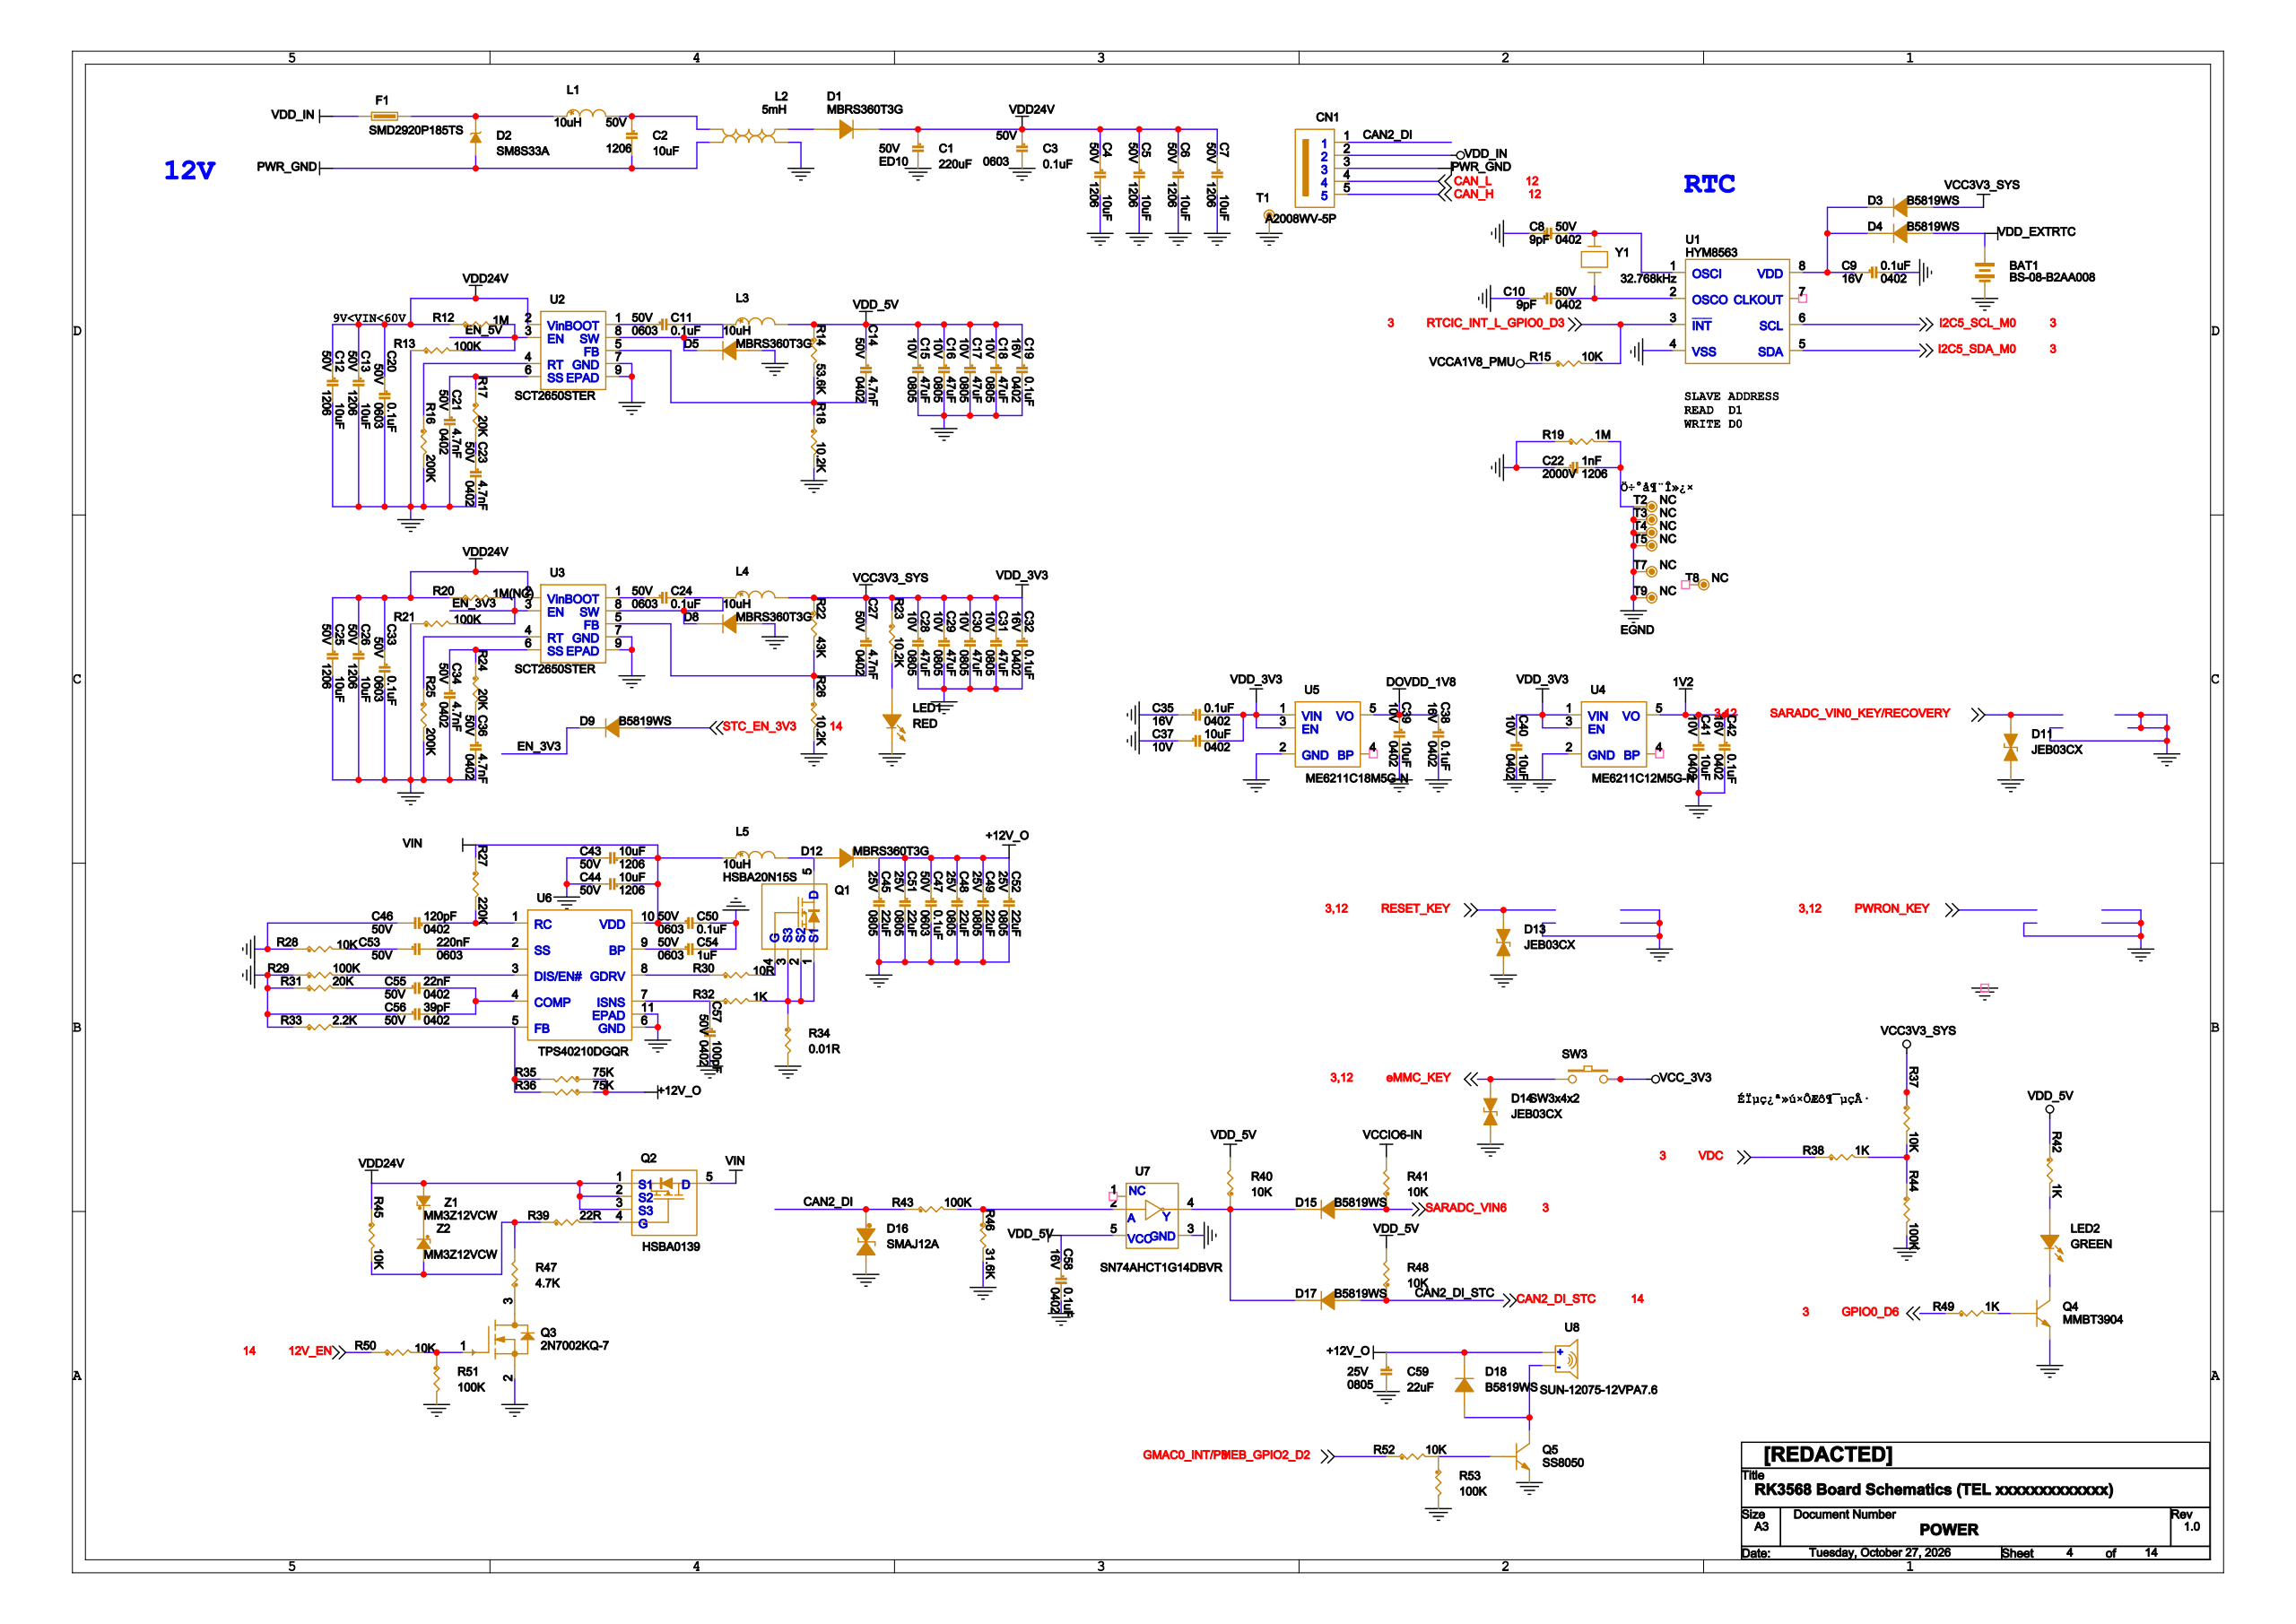Circuit board | Cadence Allegro | 669 parts | 581 nets | one sheet of the schematic
Parts on this sheet (reference | value | footprint):
BAT1 | BS-08-B2AA008 | CR2032
C1 | 220uF | ED10
C3 | 0.1uF | C0603
C4 | 10uF | C1206
C5 | 10uF | C1206
C6 | 10uF | C1206
C7 | 10uF | C1206
C8 | 9pF | C0402
C9 | 0.1uF | C0402
C10 | 9pF | C0402
C11 | 0.1uF | C0603
C12 | 10uF | C1206
C13 | 10uF | C1206
C14 | 4.7nF | C0402
C15 | 47uF | C0805
C16 | 47uF | C0805
C17 | 47uF | C0805
C18 | 47uF | C0805
C19 | 0.1uF | C0402
C20 | 0.1uF | C0603
C21 | 4.7nF | C0402
C22 | 1nF | C1206
C23 | 4.7nF | C0402
C24 | 0.1uF | C0603
C25 | 10uF | C1206
C26 | 10uF | C1206
C27 | 4.7nF | C0402
C28 | 47uF | C0805
C29 | 47uF | C0805
C30 | 47uF | C0805
C31 | 47uF | C0805
C32 | 0.1uF | C0402
C33 | 0.1uF | C0603
C34 | 4.7nF | C0402
C35 | 0.1uF | C0402
C36 | 4.7nF | C0402
C37 | 10uF | C0402
C38 | 0.1uF | C0402
C39 | 10uF | C0402
C40 | 10uF | C0402
C41 | 10uF | C0402
C42 | 0.1uF | C0402
C43 | 10uF | C1206
C44 | 10uF | C1206
C45 | 22uF | C0805
C46 | 120pF | C0402
C47 | 0.1uF | C0603
C48 | 22uF | C0805
C49 | 22uF | C0805
C50 | 0.1uF | C0603
C51 | 22uF | C0805
C52 | 22uF | C0805
C53 | 220nF | C0603
C54 | 1uF | C0603
C55 | 22nF | C0402
C56 | 39pF | C0402
C57 | 100pF | C0402
C58 | 0.1uF | C0402
C59 | 22uF | C0805
CN1 | A2008WV-5P | A2008WV_5P
D1 | MBRS360T3G | SMC
D2 | SM8S33A | DO_218AB
D3 | B5819WS | SOD323
D4 | B5819WS | SOD323
D5 | MBRS360T3G | SMC
D8 | MBRS360T3G | SMC
D9 | B5819WS | SOD323
D11 | JEB03CX | SOD323
D12 | MBRS360T3G | SMC
D13 | JEB03CX | SOD323
D14 | JEB03CX | SOD323
D15 | B5819WS | SOD323
D16 | SMAJ12A | SMA
D17 | B5819WS | SOD323
D18 | B5819WS | SOD323
F1 | SMD2920P185TS | R2920
L1 | 10uH | IND0630
L2 | 5mH | SQ1212WS
L3 | 10uH | IND0630
L4 | 10uH | IND0630
L5 | 10uH | IND0630
LED1 | RED | D0603
LED2 | GREEN | LED_0603
Q1 | HSBA20N15S | DFN5X6
Q2 | HSBA0139 | DFN5X6
Q3 | 2N7002KQ-7 | SOT-23
Q4 | MMBT3904 | SOT-23
Q5 | SS8050 | SOT-23
R12 | 1M | R0402
R13 | 100K | R0402
R14 | 53.6K | R0402
R15 | 10K | R0402
R16 | 200K | R0402
R17 | 20K | R0402
R18 | 10.2K | R0402
R19 | 1M | R1206
R20 | 1M(NC) | R0402
R21 | 100K | R0402
R22 | 43K | R0402
R23 | 10.2K | R0402
R24 | 20K | R0402
R25 | 200K | R0402
R26 | 10.2K | R0402
R27 | 220K | R0402
R28 | 10K | R0402
R29 | 100K | R0402
R30 | 10R | R0402
R31 | 20K | R0402
R32 | 1K | R0402
R33 | 2.2K | R0402
R34 | 0.01R | R2512
R35 | 75K | R0402
R36 | 75K | R0402
R37 | 10K | R0402
R38 | 1K | R0402
R39 | 22R | R0402
R40 | 10K | R0402
R41 | 10K | R0402
R42 | 1K | R0402
R43 | 100K | R0402
R44 | 100K | R0402
R45 | 10K | R0402
R46 | 31.6K | R0402
R47 | 4.7K | R0402
R48 | 10K | R0402
R49 | 1K | R0402
R50 | 10K | R0402
R51 | 100K | R0402
R52 | 10K | R0402
R53 | 100K | R0402
SW3 | SW3x4x2 | SW3X4X2
T1 | DNP | D2P2MM_3P2MM
T2 | NC | M3
T3 | NC | M3
T4 | NC | M3
T5 | NC | M3
T7 | NC | M3
T9 | NC | M3
U1 | HYM8563 | SO8
U2 | SCT2650STER | SO8_EPAD
U3 | SCT2650STER | SO8_EPAD
U4 | ME6211C12M5G-N | SOT23-5
U5 | ME6211C18M5G-N | SOT23-5
U6 | TPS40210DGQR | HVSSOP10
U7 | SN74AHCT1G14DBVR | SOT23-5
U8 | SUN-12075-12VPA7.6 | BEEP_7P6_12
Y1 | 32.768kHz | X3215
Z1 | MM3Z12VCW | SOD323
Z2 | MM3Z12VCW | SOD323
Nets of these parts (net: part-pin ...):
PWR_GND: CN1-3 D2-1 L2-4
GND: BAT1-2 C1-2 C3-2 C4-2 C5-2 C6-2 C7-2 C8-1 C9-2 C10-1 C12-2 C13-2 C15-2 C16-2 C17-2 C18-2 C19-2 C20-2 C21-2 C22-1 C23-2 C25-2 C26-2 C28-2 C29-2 C30-2 C31-2 C32-2 C33-2 C34-2 C35-1 C36-2 C37-1 C38-2 C39-2 C40-2 C41-2 C42-2 C43-2 C44-2 C45-2 C46-2 C47-2 C48-2 C49-2 C50-2 C51-2 C52-2 C54-2 C56-1 C57-2 C58-2 C59-2 D5-1 D8-1 D11-1 D13-1 D14-1 D16-1 L2-3 LED1-2 Q3-2 Q4-2 Q5-2 R13-1 R16-2 R18-2 R19-1 R21-1 R25-2 R26-2 R28-1 R29-1 R31-1 R33-1 R34-2 R44-2 R46-2 R51-2 R53-2 T1-1 U1-4 U2-7 U2-9 U3-7 U3-9 U4-2 U5-2 U6-6 U6-11 U7-3
VDD_5V: C14-1 C15-1 C16-1 C17-1 C18-1 C19-1 C58-1 L3-2 R14-1 R40-2 R42-1 R48-2 U7-5
VDD_IN: CN1-2 F1-1
STC_EN_3V3: D9-1
EN_3V3: D9-2 R20-2 R21-2 U3-3
SARADC_VIN6: D15-1 R41-1
N84697404: D15-2 D17-2 R40-1 U7-4
CAN2_DI_STC: D17-1 R48-1
VCC3V3_SYS: C27-1 C28-1 C29-1 C30-1 C31-1 C32-1 C35-2 C37-2 C40-1 D3-1 L4-2 R22-1 R23-1 R37-1 U4-1 U4-3 U5-1 U5-3
N83817809: C9-1 D3-2 D4-2 U1-8
VDD_EXTRTC: BAT1-1 D4-1
N84539976: D18-1 Q5-3 U8-2
+12V_O: C45-1 C47-1 C48-1 C49-1 C51-1 C52-1 C59-1 D12-2 D18-2 R35-1 R36-1 U8-1
12V_EN: R50-1
1V2: C41-1 C42-1 U4-5
DOVDD_1V8: C38-1 C39-1 U5-5
VCCIO6-IN: R41-2
N84487366: L1-2 L2-2
VDD24V: C1-1 C3-1 C4-1 C5-1 C6-1 C7-1 C12-1 C13-1 C20-1 C25-1 C26-1 C33-1 D1-2 Q2-1 Q2-2 Q2-3 R12-1 R20-1 R45-1 U2-2 U3-2 Z1-1
VIN: C43-1 C44-1 C50-1 L5-1 Q2-5 R27-1 U6-10
N84513302: C54-1 U6-9
N84513086: C53-1 R28-2
N84513074: C53-2 U6-2
N84501230: C11-1 U2-1
N84501232: C11-2 D5-2 L3-1 U2-8
N84502823: C24-1 U3-1
N84502825: C24-2 D8-2 L4-1 U3-8
RESET_KEY: D13-2
N83817841: C10-2 U1-2 Y1-1
N83817824: C8-2 U1-1 Y1-2
N84501270: C14-2 R14-2 R18-1 U2-5
N84501172: C21-1 R17-1 U2-6
N84501368: C23-1 R17-2
N84502863: C27-2 R22-2 R26-1 U3-5
N84502765: C34-1 R24-1 U3-6
N84502969: C36-1 R24-2
EGND: C22-2 R19-2 T2-1 T3-1 T4-1 T5-1 T7-1 T9-1
N84513062: C46-1 R27-2 U6-1
CAN_L: CN1-4
CAN_H: CN1-5
N84518896: C55-1 R31-2
N84513146: C55-2 C56-2 U6-4
N84513390: C57-1 R32-1 U6-7
CAN2_DI: CN1-1 D16-2 R43-1
N84487324: D2-2 F1-2 L1-1
SARADC_VIN0_KEY/RECOVERY: D11-2
EMMC_KEY: D14-2 SW3-1
N84513459: D12-1 L5-2 Q1-5
N84487390: D1-1 L2-1
N84503640: LED1-1 R23-2
VCC_3V3: SW3-2
N84513114: Q3-1 R50-2 R51-1
N845290030: Q3-3 R47-1
N84536886: Q2-4 R39-2
N84539956: Q5-1 R52-2 R53-1
EN_5V: R12-2 R13-2 U2-3
N84536862: R39-1 R45-2 R47-2 Z2-1
VCCA1V8_PMU: R15-1
RTCIC_INT_L_GPIO0_D3: R15-2 U1-3
N83814596: R37-2 R38-2 R44-1
GMAC0_INT/PMEB_GPIO2_D2: R52-1
N84697410: R43-2 R46-1 U7-2
N84513084: R29-2 U6-3
N84513428: Q1-1 Q1-2 Q1-3 R32-2 R34-1
VDC: R38-1
N84255296: LED2-1 R42-2
GPIO0_D6: R49-1
N83966565: Q4-1 R49-2
N84501168: R16-1 U2-4
N84502761: R25-1 U3-4
N84513404: R30-1 U6-8
N84513432: Q1-4 R30-2
I2C5_SCL_M0: U1-6
I2C5_SDA_M0: U1-5
N84513200: R33-2 R35-2 R36-2 U6-5
N845368291: Z1-2 Z2-2
N83967011: LED2-2 Q4-3